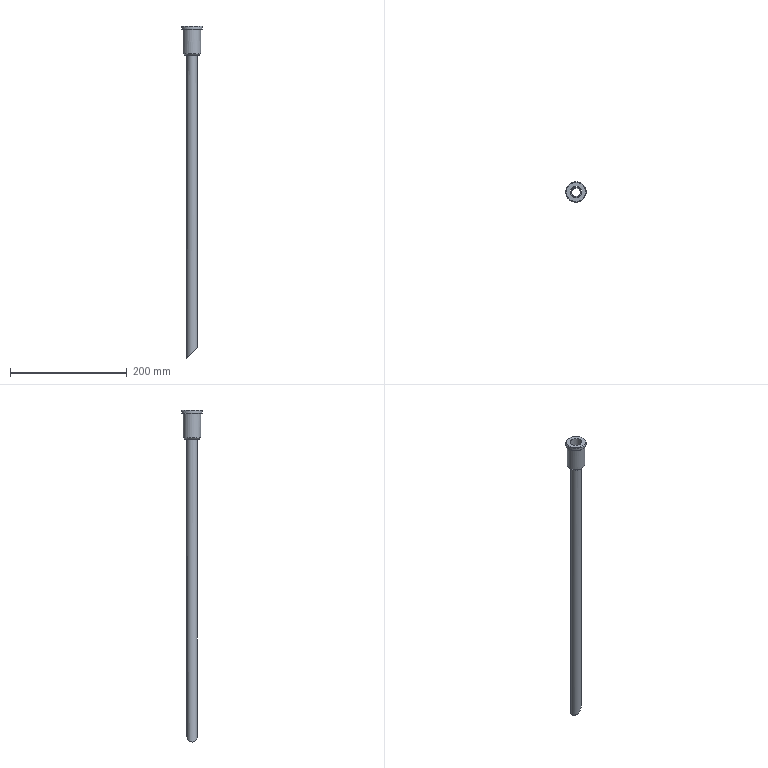Part | STEP file | HL4GZ-1.581.020 (return pipe weldment) | 2 solids | 14 faces | box 35 x 35 x 570 mm | volume 62212 mm3 | plane 5 | cylinder 5 | cone 3 | torus 1 | commonest cylinder face diameters 15 x1 18 x1 20 x1 30 x1 35 x1
STEP:
#1=CARTESIAN_POINT('',(0.,0.,0.));
#2=DIRECTION('',(0.,0.,1.));
#3=DIRECTION('',(1.,0.,0.));
#4=AXIS2_PLACEMENT_3D('',#1,#2,#3);
#5=CARTESIAN_POINT('',(1972.5,-700.,-232.5));
#6=VERTEX_POINT('',#5);
#7=CARTESIAN_POINT('',(1965.,-692.5,-240.));
#8=VERTEX_POINT('',#7);
#9=CARTESIAN_POINT('',(1965.,-700.,-240.));
#10=DIRECTION('',(0.7071,0.,-0.7071));
#11=DIRECTION('',(0.7071,0.,0.7071));
#12=AXIS2_PLACEMENT_3D('',#9,#10,#11);
#13=ELLIPSE('',#12,10.607,7.5);
#14=CARTESIAN_POINT('',(1970.142,-684.,-234.858));
#15=DIRECTION('',(0.7071,0.,-0.7071));
#16=DIRECTION('',(0.7071,0.,0.7071));
#17=AXIS2_PLACEMENT_3D('',#14,#15,#16);
#18=PLANE('',#17);
#19=CARTESIAN_POINT('',(-7.272,16.));
#20=DIRECTION('',(1.,0.));
#21=AXIS2_PLACEMENT_2D('',#19,#20);
#22=ELLIPSE('',#21,10.607,7.5);
#23=(GEOMETRIC_REPRESENTATION_CONTEXT(2)PARAMETRIC_REPRESENTATION_CONTEXT()REPRESENTATION_CONTEXT('',''));
#24=DEFINITIONAL_REPRESENTATION('',(#22),#23);
#25=PCURVE('',#18,#24);
#26=CARTESIAN_POINT('',(1965.,-700.,311.));
#27=DIRECTION('',(0.,0.,1.));
#28=DIRECTION('',(0.,1.,0.));
#29=AXIS2_PLACEMENT_3D('',#26,#27,#28);
#30=CYLINDRICAL_SURFACE('',#29,7.5);
#31=CARTESIAN_POINT('',(4.712,-543.5));
#32=CARTESIAN_POINT('',(4.617,-543.496));
#33=CARTESIAN_POINT('',(4.427,-543.707));
#34=CARTESIAN_POINT('',(4.141,-544.604));
#35=CARTESIAN_POINT('',(3.856,-546.021));
#36=CARTESIAN_POINT('',(3.57,-547.842));
#37=CARTESIAN_POINT('',(3.284,-549.918));
#38=CARTESIAN_POINT('',(2.999,-552.082));
#39=CARTESIAN_POINT('',(2.713,-554.158));
#40=CARTESIAN_POINT('',(2.428,-555.979));
#41=CARTESIAN_POINT('',(2.142,-557.396));
#42=CARTESIAN_POINT('',(1.856,-558.295));
#43=CARTESIAN_POINT('',(1.571,-558.603));
#44=CARTESIAN_POINT('',(1.285,-558.295));
#45=CARTESIAN_POINT('',(0.9996,-557.396));
#46=CARTESIAN_POINT('',(0.714,-555.979));
#47=CARTESIAN_POINT('',(0.4284,-554.158));
#48=CARTESIAN_POINT('',(0.1428,-552.082));
#49=CARTESIAN_POINT('',(-0.1428,-549.918));
#50=CARTESIAN_POINT('',(-0.4284,-547.842));
#51=CARTESIAN_POINT('',(-0.714,-546.021));
#52=CARTESIAN_POINT('',(-0.9996,-544.604));
#53=CARTESIAN_POINT('',(-1.285,-543.707));
#54=CARTESIAN_POINT('',(-1.476,-543.496));
#55=CARTESIAN_POINT('',(-1.571,-543.5));
#56=B_SPLINE_CURVE_WITH_KNOTS('',3,(#31,#32,#33,#34,#35,#36,#37,#38,#39,#40,#41,#42,#43,#44,#45,#46,#47,#48,#49,#50,#51,#52,#53,#54,#55),.UNSPECIFIED.,.F.,.F.,(4,1,1,1,1,1,1,1,1,1,1,1,1,1,1,1,1,1,1,1,1,1,4),(0.,0.2856,0.5712,0.8568,1.142,1.428,1.714,1.999,2.285,2.57,2.856,3.142,3.427,3.713,3.998,4.284,4.57,4.855,5.141,5.426,5.712,5.998,6.283),.QUASI_UNIFORM_KNOTS.);
#57=(GEOMETRIC_REPRESENTATION_CONTEXT(2)PARAMETRIC_REPRESENTATION_CONTEXT()REPRESENTATION_CONTEXT('',''));
#58=DEFINITIONAL_REPRESENTATION('',(#56),#57);
#59=PCURVE('',#30,#58);
#60=SURFACE_CURVE('',#13,(#25,#59),.PCURVE_S1.);
#61=EDGE_CURVE('',#6,#8,#60,.T.);
#62=ORIENTED_EDGE('',*,*,#61,.F.);
#63=CARTESIAN_POINT('',(1965.,-700.,-240.));
#64=DIRECTION('',(0.7071,0.,-0.7071));
#65=DIRECTION('',(0.7071,0.,0.7071));
#66=AXIS2_PLACEMENT_3D('',#63,#64,#65);
#67=ELLIPSE('',#66,10.607,7.5);
#68=CARTESIAN_POINT('',(-7.272,16.));
#69=DIRECTION('',(1.,0.));
#70=AXIS2_PLACEMENT_2D('',#68,#69);
#71=ELLIPSE('',#70,10.607,7.5);
#72=(GEOMETRIC_REPRESENTATION_CONTEXT(2)PARAMETRIC_REPRESENTATION_CONTEXT()REPRESENTATION_CONTEXT('',''));
#73=DEFINITIONAL_REPRESENTATION('',(#71),#72);
#74=PCURVE('',#18,#73);
#75=CARTESIAN_POINT('',(10.996,-543.5));
#76=CARTESIAN_POINT('',(10.9,-543.496));
#77=CARTESIAN_POINT('',(10.71,-543.707));
#78=CARTESIAN_POINT('',(10.424,-544.604));
#79=CARTESIAN_POINT('',(10.139,-546.021));
#80=CARTESIAN_POINT('',(9.853,-547.842));
#81=CARTESIAN_POINT('',(9.568,-549.918));
#82=CARTESIAN_POINT('',(9.282,-552.082));
#83=CARTESIAN_POINT('',(8.996,-554.158));
#84=CARTESIAN_POINT('',(8.711,-555.979));
#85=CARTESIAN_POINT('',(8.425,-557.396));
#86=CARTESIAN_POINT('',(8.14,-558.295));
#87=CARTESIAN_POINT('',(7.854,-558.603));
#88=CARTESIAN_POINT('',(7.568,-558.295));
#89=CARTESIAN_POINT('',(7.283,-557.396));
#90=CARTESIAN_POINT('',(6.997,-555.979));
#91=CARTESIAN_POINT('',(6.712,-554.158));
#92=CARTESIAN_POINT('',(6.426,-552.082));
#93=CARTESIAN_POINT('',(6.14,-549.918));
#94=CARTESIAN_POINT('',(5.855,-547.842));
#95=CARTESIAN_POINT('',(5.569,-546.021));
#96=CARTESIAN_POINT('',(5.284,-544.604));
#97=CARTESIAN_POINT('',(4.998,-543.707));
#98=CARTESIAN_POINT('',(4.808,-543.496));
#99=CARTESIAN_POINT('',(4.712,-543.5));
#100=B_SPLINE_CURVE_WITH_KNOTS('',3,(#75,#76,#77,#78,#79,#80,#81,#82,#83,#84,#85,#86,#87,#88,#89,#90,#91,#92,#93,#94,#95,#96,#97,#98,#99),.UNSPECIFIED.,.F.,.F.,(4,1,1,1,1,1,1,1,1,1,1,1,1,1,1,1,1,1,1,1,1,1,4),(0.,0.2856,0.5712,0.8568,1.142,1.428,1.714,1.999,2.285,2.57,2.856,3.142,3.427,3.713,3.998,4.284,4.57,4.855,5.141,5.426,5.712,5.998,6.283),.QUASI_UNIFORM_KNOTS.);
#101=(GEOMETRIC_REPRESENTATION_CONTEXT(2)PARAMETRIC_REPRESENTATION_CONTEXT()REPRESENTATION_CONTEXT('',''));
#102=DEFINITIONAL_REPRESENTATION('',(#100),#101);
#103=PCURVE('',#30,#102);
#104=SURFACE_CURVE('',#67,(#74,#103),.PCURVE_S1.);
#105=EDGE_CURVE('',#8,#6,#104,.T.);
#106=ORIENTED_EDGE('',*,*,#105,.F.);
#107=EDGE_LOOP('',(#62,#106));
#108=FACE_BOUND('',#107,.T.);
#109=CARTESIAN_POINT('',(1974.,-700.,-231.));
#110=VERTEX_POINT('',#109);
#111=CARTESIAN_POINT('',(1965.,-691.,-240.));
#112=VERTEX_POINT('',#111);
#113=CARTESIAN_POINT('',(1965.,-700.,-240.));
#114=DIRECTION('',(-0.7071,0.,0.7071));
#115=DIRECTION('',(0.7071,0.,0.7071));
#116=AXIS2_PLACEMENT_3D('',#113,#114,#115);
#117=ELLIPSE('',#116,12.728,9.);
#118=CARTESIAN_POINT('',(5.456,16.));
#119=CARTESIAN_POINT('',(5.456,0.4115));
#120=CARTESIAN_POINT('',(-13.636,8.206));
#121=CARTESIAN_POINT('',(-32.728,16.));
#122=CARTESIAN_POINT('',(-13.636,23.794));
#123=CARTESIAN_POINT('',(5.456,31.588));
#124=CARTESIAN_POINT('',(5.456,16.));
#125=(BOUNDED_CURVE()B_SPLINE_CURVE(2,(#118,#119,#120,#121,#122,#123,#124),.UNSPECIFIED.,.T.,.F.)B_SPLINE_CURVE_WITH_KNOTS((1,2,2,2,2,1),(-2.094,0.,2.094,4.189,6.283,8.378),.UNSPECIFIED.)CURVE()GEOMETRIC_REPRESENTATION_ITEM()RATIONAL_B_SPLINE_CURVE((1.,0.5,1.,0.5,1.,0.5,1.))REPRESENTATION_ITEM(''));
#126=(GEOMETRIC_REPRESENTATION_CONTEXT(2)PARAMETRIC_REPRESENTATION_CONTEXT()REPRESENTATION_CONTEXT('',''));
#127=DEFINITIONAL_REPRESENTATION('',(#125),#126);
#128=PCURVE('',#18,#127);
#129=CARTESIAN_POINT('',(1965.,-700.,311.));
#130=DIRECTION('',(0.,0.,1.));
#131=DIRECTION('',(0.,1.,0.));
#132=AXIS2_PLACEMENT_3D('',#129,#130,#131);
#133=CYLINDRICAL_SURFACE('',#132,9.);
#134=CARTESIAN_POINT('',(4.712,-542.));
#135=CARTESIAN_POINT('',(4.808,-541.995));
#136=CARTESIAN_POINT('',(4.998,-542.249));
#137=CARTESIAN_POINT('',(5.284,-543.325));
#138=CARTESIAN_POINT('',(5.569,-545.026));
#139=CARTESIAN_POINT('',(5.855,-547.21));
#140=CARTESIAN_POINT('',(6.14,-549.702));
#141=CARTESIAN_POINT('',(6.426,-552.298));
#142=CARTESIAN_POINT('',(6.712,-554.79));
#143=CARTESIAN_POINT('',(6.997,-556.974));
#144=CARTESIAN_POINT('',(7.283,-558.675));
#145=CARTESIAN_POINT('',(7.568,-559.754));
#146=CARTESIAN_POINT('',(7.854,-560.123));
#147=CARTESIAN_POINT('',(8.14,-559.754));
#148=CARTESIAN_POINT('',(8.425,-558.675));
#149=CARTESIAN_POINT('',(8.711,-556.974));
#150=CARTESIAN_POINT('',(8.996,-554.79));
#151=CARTESIAN_POINT('',(9.282,-552.298));
#152=CARTESIAN_POINT('',(9.568,-549.702));
#153=CARTESIAN_POINT('',(9.853,-547.21));
#154=CARTESIAN_POINT('',(10.139,-545.026));
#155=CARTESIAN_POINT('',(10.424,-543.325));
#156=CARTESIAN_POINT('',(10.71,-542.249));
#157=CARTESIAN_POINT('',(10.9,-541.995));
#158=CARTESIAN_POINT('',(10.996,-542.));
#159=B_SPLINE_CURVE_WITH_KNOTS('',3,(#134,#135,#136,#137,#138,#139,#140,#141,#142,#143,#144,#145,#146,#147,#148,#149,#150,#151,#152,#153,#154,#155,#156,#157,#158),.UNSPECIFIED.,.F.,.F.,(4,1,1,1,1,1,1,1,1,1,1,1,1,1,1,1,1,1,1,1,1,1,4),(0.,0.2856,0.5712,0.8568,1.142,1.428,1.714,1.999,2.285,2.57,2.856,3.142,3.427,3.713,3.998,4.284,4.57,4.855,5.141,5.426,5.712,5.998,6.283),.QUASI_UNIFORM_KNOTS.);
#160=(GEOMETRIC_REPRESENTATION_CONTEXT(2)PARAMETRIC_REPRESENTATION_CONTEXT()REPRESENTATION_CONTEXT('',''));
#161=DEFINITIONAL_REPRESENTATION('',(#159),#160);
#162=PCURVE('',#133,#161);
#163=SURFACE_CURVE('',#117,(#128,#162),.PCURVE_S1.);
#164=EDGE_CURVE('',#110,#112,#163,.T.);
#165=ORIENTED_EDGE('',*,*,#164,.F.);
#166=CARTESIAN_POINT('',(1965.,-700.,-240.));
#167=DIRECTION('',(-0.7071,0.,0.7071));
#168=DIRECTION('',(0.7071,0.,0.7071));
#169=AXIS2_PLACEMENT_3D('',#166,#167,#168);
#170=ELLIPSE('',#169,12.728,9.);
#171=CARTESIAN_POINT('',(5.456,16.));
#172=CARTESIAN_POINT('',(5.456,0.4115));
#173=CARTESIAN_POINT('',(-13.636,8.206));
#174=CARTESIAN_POINT('',(-32.728,16.));
#175=CARTESIAN_POINT('',(-13.636,23.794));
#176=CARTESIAN_POINT('',(5.456,31.588));
#177=CARTESIAN_POINT('',(5.456,16.));
#178=(BOUNDED_CURVE()B_SPLINE_CURVE(2,(#171,#172,#173,#174,#175,#176,#177),.UNSPECIFIED.,.T.,.F.)B_SPLINE_CURVE_WITH_KNOTS((1,2,2,2,2,1),(-2.094,0.,2.094,4.189,6.283,8.378),.UNSPECIFIED.)CURVE()GEOMETRIC_REPRESENTATION_ITEM()RATIONAL_B_SPLINE_CURVE((1.,0.5,1.,0.5,1.,0.5,1.))REPRESENTATION_ITEM(''));
#179=(GEOMETRIC_REPRESENTATION_CONTEXT(2)PARAMETRIC_REPRESENTATION_CONTEXT()REPRESENTATION_CONTEXT('',''));
#180=DEFINITIONAL_REPRESENTATION('',(#178),#179);
#181=PCURVE('',#18,#180);
#182=CARTESIAN_POINT('',(-1.571,-542.));
#183=CARTESIAN_POINT('',(-1.476,-541.995));
#184=CARTESIAN_POINT('',(-1.285,-542.249));
#185=CARTESIAN_POINT('',(-0.9996,-543.325));
#186=CARTESIAN_POINT('',(-0.714,-545.026));
#187=CARTESIAN_POINT('',(-0.4284,-547.21));
#188=CARTESIAN_POINT('',(-0.1428,-549.702));
#189=CARTESIAN_POINT('',(0.1428,-552.298));
#190=CARTESIAN_POINT('',(0.4284,-554.79));
#191=CARTESIAN_POINT('',(0.714,-556.974));
#192=CARTESIAN_POINT('',(0.9996,-558.675));
#193=CARTESIAN_POINT('',(1.285,-559.754));
#194=CARTESIAN_POINT('',(1.571,-560.123));
#195=CARTESIAN_POINT('',(1.856,-559.754));
#196=CARTESIAN_POINT('',(2.142,-558.675));
#197=CARTESIAN_POINT('',(2.428,-556.974));
#198=CARTESIAN_POINT('',(2.713,-554.79));
#199=CARTESIAN_POINT('',(2.999,-552.298));
#200=CARTESIAN_POINT('',(3.284,-549.702));
#201=CARTESIAN_POINT('',(3.57,-547.21));
#202=CARTESIAN_POINT('',(3.856,-545.026));
#203=CARTESIAN_POINT('',(4.141,-543.325));
#204=CARTESIAN_POINT('',(4.427,-542.249));
#205=CARTESIAN_POINT('',(4.617,-541.995));
#206=CARTESIAN_POINT('',(4.712,-542.));
#207=B_SPLINE_CURVE_WITH_KNOTS('',3,(#182,#183,#184,#185,#186,#187,#188,#189,#190,#191,#192,#193,#194,#195,#196,#197,#198,#199,#200,#201,#202,#203,#204,#205,#206),.UNSPECIFIED.,.F.,.F.,(4,1,1,1,1,1,1,1,1,1,1,1,1,1,1,1,1,1,1,1,1,1,4),(0.,0.2856,0.5712,0.8568,1.142,1.428,1.714,1.999,2.285,2.57,2.856,3.142,3.427,3.713,3.998,4.284,4.57,4.855,5.141,5.426,5.712,5.998,6.283),.QUASI_UNIFORM_KNOTS.);
#208=(GEOMETRIC_REPRESENTATION_CONTEXT(2)PARAMETRIC_REPRESENTATION_CONTEXT()REPRESENTATION_CONTEXT('',''));
#209=DEFINITIONAL_REPRESENTATION('',(#207),#208);
#210=PCURVE('',#133,#209);
#211=SURFACE_CURVE('',#170,(#181,#210),.PCURVE_S1.);
#212=EDGE_CURVE('',#112,#110,#211,.T.);
#213=ORIENTED_EDGE('',*,*,#212,.F.);
#214=EDGE_LOOP('',(#165,#213));
#215=FACE_BOUND('',#214,.T.);
#216=ADVANCED_FACE('',(#108,#215),#18,.T.);
#217=CARTESIAN_POINT('',(1965.,-692.5,291.));
#218=VERTEX_POINT('',#217);
#219=CARTESIAN_POINT('',(1965.,-700.,291.));
#220=DIRECTION('',(0.,0.,1.));
#221=DIRECTION('',(0.,1.,0.));
#222=AXIS2_PLACEMENT_3D('',#219,#220,#221);
#223=CIRCLE('',#222,7.5);
#224=CARTESIAN_POINT('',(1965.,-700.,291.));
#225=DIRECTION('',(0.,0.,-1.));
#226=DIRECTION('',(-1.,0.,0.));
#227=AXIS2_PLACEMENT_3D('',#224,#225,#226);
#228=PLANE('',#227);
#229=CARTESIAN_POINT('',(0.,7.5));
#230=CARTESIAN_POINT('',(12.99,7.5));
#231=CARTESIAN_POINT('',(6.495,-3.75));
#232=CARTESIAN_POINT('',(0.,-15.));
#233=CARTESIAN_POINT('',(-6.495,-3.75));
#234=CARTESIAN_POINT('',(-12.99,7.5));
#235=CARTESIAN_POINT('',(0.,7.5));
#236=(BOUNDED_CURVE()B_SPLINE_CURVE(2,(#229,#230,#231,#232,#233,#234,#235),.UNSPECIFIED.,.T.,.F.)B_SPLINE_CURVE_WITH_KNOTS((1,2,2,2,2,1),(-2.094,0.,2.094,4.189,6.283,8.378),.UNSPECIFIED.)CURVE()GEOMETRIC_REPRESENTATION_ITEM()RATIONAL_B_SPLINE_CURVE((1.,0.5,1.,0.5,1.,0.5,1.))REPRESENTATION_ITEM(''));
#237=(GEOMETRIC_REPRESENTATION_CONTEXT(2)PARAMETRIC_REPRESENTATION_CONTEXT()REPRESENTATION_CONTEXT('',''));
#238=DEFINITIONAL_REPRESENTATION('',(#236),#237);
#239=PCURVE('',#228,#238);
#240=CARTESIAN_POINT('',(0.,-20.));
#241=DIRECTION('',(1.,0.));
#242=VECTOR('',#241,1.);
#243=LINE('',#240,#242);
#244=(GEOMETRIC_REPRESENTATION_CONTEXT(2)PARAMETRIC_REPRESENTATION_CONTEXT()REPRESENTATION_CONTEXT('',''));
#245=DEFINITIONAL_REPRESENTATION('',(#243),#244);
#246=PCURVE('',#30,#245);
#247=SURFACE_CURVE('',#223,(#239,#246),.PCURVE_S1.);
#248=EDGE_CURVE('',#218,#218,#247,.T.);
#249=ORIENTED_EDGE('',*,*,#248,.F.);
#250=EDGE_LOOP('',(#249));
#251=FACE_BOUND('',#250,.T.);
#252=CARTESIAN_POINT('',(1965.,-691.,291.));
#253=VERTEX_POINT('',#252);
#254=CARTESIAN_POINT('',(1965.,-700.,291.));
#255=DIRECTION('',(0.,0.,-1.));
#256=DIRECTION('',(0.,1.,0.));
#257=AXIS2_PLACEMENT_3D('',#254,#255,#256);
#258=CIRCLE('',#257,9.);
#259=CARTESIAN_POINT('',(0.,0.));
#260=DIRECTION('',(0.,1.));
#261=AXIS2_PLACEMENT_2D('',#259,#260);
#262=CIRCLE('',#261,9.);
#263=(GEOMETRIC_REPRESENTATION_CONTEXT(2)PARAMETRIC_REPRESENTATION_CONTEXT()REPRESENTATION_CONTEXT('',''));
#264=DEFINITIONAL_REPRESENTATION('',(#262),#263);
#265=PCURVE('',#228,#264);
#266=CARTESIAN_POINT('',(6.283,-20.));
#267=DIRECTION('',(-1.,0.));
#268=VECTOR('',#267,1.);
#269=LINE('',#266,#268);
#270=(GEOMETRIC_REPRESENTATION_CONTEXT(2)PARAMETRIC_REPRESENTATION_CONTEXT()REPRESENTATION_CONTEXT('',''));
#271=DEFINITIONAL_REPRESENTATION('',(#269),#270);
#272=PCURVE('',#133,#271);
#273=SURFACE_CURVE('',#258,(#265,#272),.PCURVE_S1.);
#274=EDGE_CURVE('',#253,#253,#273,.T.);
#275=ORIENTED_EDGE('',*,*,#274,.F.);
#276=EDGE_LOOP('',(#275));
#277=FACE_BOUND('',#276,.T.);
#278=ADVANCED_FACE('',(#251,#277),#228,.F.);
#279=ORIENTED_EDGE('',*,*,#105,.F.);
#280=CARTESIAN_POINT('',(1965.,-692.5,-240.));
#281=CARTESIAN_POINT('',(1965.,-692.5,291.));
#282=B_SPLINE_CURVE_WITH_KNOTS('',1,(#280,#281),.UNSPECIFIED.,.F.,.F.,(2,2),(-551.,-20.),.PIECEWISE_BEZIER_KNOTS.);
#283=CARTESIAN_POINT('',(6.283,0.));
#284=DIRECTION('',(0.,1.));
#285=VECTOR('',#284,1.);
#286=LINE('',#283,#285);
#287=(GEOMETRIC_REPRESENTATION_CONTEXT(2)PARAMETRIC_REPRESENTATION_CONTEXT()REPRESENTATION_CONTEXT('',''));
#288=DEFINITIONAL_REPRESENTATION('',(#286),#287);
#289=PCURVE('',#30,#288);
#290=CARTESIAN_POINT('',(0.,0.));
#291=DIRECTION('',(0.,1.));
#292=VECTOR('',#291,1.);
#293=LINE('',#290,#292);
#294=(GEOMETRIC_REPRESENTATION_CONTEXT(2)PARAMETRIC_REPRESENTATION_CONTEXT()REPRESENTATION_CONTEXT('',''));
#295=DEFINITIONAL_REPRESENTATION('',(#293),#294);
#296=PCURVE('',#30,#295);
#297=SEAM_CURVE('',#282,(#289,#296),.PCURVE_S1.);
#298=EDGE_CURVE('',#8,#218,#297,.T.);
#299=ORIENTED_EDGE('',*,*,#298,.T.);
#300=ORIENTED_EDGE('',*,*,#248,.F.);
#301=ORIENTED_EDGE('',*,*,#298,.F.);
#302=ORIENTED_EDGE('',*,*,#61,.F.);
#303=EDGE_LOOP('',(#279,#299,#300,#301,#302));
#304=FACE_BOUND('',#303,.F.);
#305=ADVANCED_FACE('',(#304),#30,.F.);
#306=ORIENTED_EDGE('',*,*,#164,.T.);
#307=CARTESIAN_POINT('',(1965.,-691.,-240.));
#308=CARTESIAN_POINT('',(1965.,-691.,291.));
#309=B_SPLINE_CURVE_WITH_KNOTS('',1,(#307,#308),.UNSPECIFIED.,.F.,.F.,(2,2),(-551.,-20.),.PIECEWISE_BEZIER_KNOTS.);
#310=CARTESIAN_POINT('',(6.283,0.));
#311=DIRECTION('',(0.,1.));
#312=VECTOR('',#311,1.);
#313=LINE('',#310,#312);
#314=(GEOMETRIC_REPRESENTATION_CONTEXT(2)PARAMETRIC_REPRESENTATION_CONTEXT()REPRESENTATION_CONTEXT('',''));
#315=DEFINITIONAL_REPRESENTATION('',(#313),#314);
#316=PCURVE('',#133,#315);
#317=CARTESIAN_POINT('',(0.,0.));
#318=DIRECTION('',(0.,1.));
#319=VECTOR('',#318,1.);
#320=LINE('',#317,#319);
#321=(GEOMETRIC_REPRESENTATION_CONTEXT(2)PARAMETRIC_REPRESENTATION_CONTEXT()REPRESENTATION_CONTEXT('',''));
#322=DEFINITIONAL_REPRESENTATION('',(#320),#321);
#323=PCURVE('',#133,#322);
#324=SEAM_CURVE('',#309,(#316,#323),.PCURVE_S1.);
#325=EDGE_CURVE('',#112,#253,#324,.T.);
#326=ORIENTED_EDGE('',*,*,#325,.T.);
#327=ORIENTED_EDGE('',*,*,#274,.T.);
#328=ORIENTED_EDGE('',*,*,#325,.F.);
#329=ORIENTED_EDGE('',*,*,#212,.T.);
#330=EDGE_LOOP('',(#306,#326,#327,#328,#329));
#331=FACE_BOUND('',#330,.T.);
#332=ADVANCED_FACE('',(#331),#133,.T.);
#333=CLOSED_SHELL('',(#216,#278,#305,#332));
#334=MANIFOLD_SOLID_BREP('',#333);
#335=CARTESIAN_POINT('',(1950.,-700.,273.));
#336=VERTEX_POINT('',#335);
#337=CARTESIAN_POINT('',(1980.,-700.,273.));
#338=VERTEX_POINT('',#337);
#339=CARTESIAN_POINT('',(1965.,-700.,273.));
#340=DIRECTION('',(0.,0.,1.));
#341=DIRECTION('',(1.,0.,0.));
#342=AXIS2_PLACEMENT_3D('',#339,#340,#341);
#343=CIRCLE('',#342,15.);
#344=CARTESIAN_POINT('',(1965.,-700.,273.));
#345=DIRECTION('',(0.,0.,1.));
#346=DIRECTION('',(-1.,0.,0.));
#347=AXIS2_PLACEMENT_3D('',#344,#345,#346);
#348=CONICAL_SURFACE('',#347,15.,0.7854);
#349=CARTESIAN_POINT('',(-3.142,0.));
#350=DIRECTION('',(1.,0.));
#351=VECTOR('',#350,1.);
#352=LINE('',#349,#351);
#353=(GEOMETRIC_REPRESENTATION_CONTEXT(2)PARAMETRIC_REPRESENTATION_CONTEXT()REPRESENTATION_CONTEXT('',''));
#354=DEFINITIONAL_REPRESENTATION('',(#352),#353);
#355=PCURVE('',#348,#354);
#356=CARTESIAN_POINT('',(1965.,-700.,315.));
#357=DIRECTION('',(0.,0.,-1.));
#358=DIRECTION('',(-1.,0.,0.));
#359=AXIS2_PLACEMENT_3D('',#356,#357,#358);
#360=CYLINDRICAL_SURFACE('',#359,15.);
#361=CARTESIAN_POINT('',(9.425,42.));
#362=DIRECTION('',(-1.,0.));
#363=VECTOR('',#362,1.);
#364=LINE('',#361,#363);
#365=(GEOMETRIC_REPRESENTATION_CONTEXT(2)PARAMETRIC_REPRESENTATION_CONTEXT()REPRESENTATION_CONTEXT('',''));
#366=DEFINITIONAL_REPRESENTATION('',(#364),#365);
#367=PCURVE('',#360,#366);
#368=SURFACE_CURVE('',#343,(#355,#367),.PCURVE_S1.);
#369=EDGE_CURVE('',#336,#338,#368,.T.);
#370=ORIENTED_EDGE('',*,*,#369,.F.);
#371=CARTESIAN_POINT('',(1952.,-700.,271.));
#372=VERTEX_POINT('',#371);
#373=CARTESIAN_POINT('',(1952.,-700.,271.));
#374=CARTESIAN_POINT('',(1950.,-700.,273.));
#375=B_SPLINE_CURVE_WITH_KNOTS('',1,(#373,#374),.UNSPECIFIED.,.F.,.F.,(2,2),(-2.828,0.),.PIECEWISE_BEZIER_KNOTS.);
#376=CARTESIAN_POINT('',(0.,0.));
#377=DIRECTION('',(0.,1.));
#378=VECTOR('',#377,1.);
#379=LINE('',#376,#378);
#380=(GEOMETRIC_REPRESENTATION_CONTEXT(2)PARAMETRIC_REPRESENTATION_CONTEXT()REPRESENTATION_CONTEXT('',''));
#381=DEFINITIONAL_REPRESENTATION('',(#379),#380);
#382=PCURVE('',#348,#381);
#383=CARTESIAN_POINT('',(6.283,0.));
#384=DIRECTION('',(0.,1.));
#385=VECTOR('',#384,1.);
#386=LINE('',#383,#385);
#387=(GEOMETRIC_REPRESENTATION_CONTEXT(2)PARAMETRIC_REPRESENTATION_CONTEXT()REPRESENTATION_CONTEXT('',''));
#388=DEFINITIONAL_REPRESENTATION('',(#386),#387);
#389=PCURVE('',#348,#388);
#390=SEAM_CURVE('',#375,(#382,#389),.PCURVE_S1.);
#391=EDGE_CURVE('',#372,#336,#390,.T.);
#392=ORIENTED_EDGE('',*,*,#391,.F.);
#393=CARTESIAN_POINT('',(1965.,-700.,271.));
#394=DIRECTION('',(0.,0.,-1.));
#395=DIRECTION('',(-1.,0.,0.));
#396=AXIS2_PLACEMENT_3D('',#393,#394,#395);
#397=CIRCLE('',#396,13.);
#398=CARTESIAN_POINT('',(6.283,-2.));
#399=DIRECTION('',(-1.,0.));
#400=VECTOR('',#399,1.);
#401=LINE('',#398,#400);
#402=(GEOMETRIC_REPRESENTATION_CONTEXT(2)PARAMETRIC_REPRESENTATION_CONTEXT()REPRESENTATION_CONTEXT('',''));
#403=DEFINITIONAL_REPRESENTATION('',(#401),#402);
#404=PCURVE('',#348,#403);
#405=CARTESIAN_POINT('',(1965.,-700.,271.));
#406=DIRECTION('',(0.,0.,-1.));
#407=DIRECTION('',(-1.,0.,0.));
#408=AXIS2_PLACEMENT_3D('',#405,#406,#407);
#409=PLANE('',#408);
#410=CARTESIAN_POINT('',(0.,0.));
#411=DIRECTION('',(1.,0.));
#412=AXIS2_PLACEMENT_2D('',#410,#411);
#413=CIRCLE('',#412,13.);
#414=(GEOMETRIC_REPRESENTATION_CONTEXT(2)PARAMETRIC_REPRESENTATION_CONTEXT()REPRESENTATION_CONTEXT('',''));
#415=DEFINITIONAL_REPRESENTATION('',(#413),#414);
#416=PCURVE('',#409,#415);
#417=SURFACE_CURVE('',#397,(#404,#416),.PCURVE_S1.);
#418=EDGE_CURVE('',#372,#372,#417,.T.);
#419=ORIENTED_EDGE('',*,*,#418,.F.);
#420=ORIENTED_EDGE('',*,*,#391,.T.);
#421=CARTESIAN_POINT('',(1965.,-700.,273.));
#422=DIRECTION('',(0.,0.,1.));
#423=DIRECTION('',(1.,0.,0.));
#424=AXIS2_PLACEMENT_3D('',#421,#422,#423);
#425=CIRCLE('',#424,15.);
#426=CARTESIAN_POINT('',(3.142,0.));
#427=DIRECTION('',(1.,0.));
#428=VECTOR('',#427,1.);
#429=LINE('',#426,#428);
#430=(GEOMETRIC_REPRESENTATION_CONTEXT(2)PARAMETRIC_REPRESENTATION_CONTEXT()REPRESENTATION_CONTEXT('',''));
#431=DEFINITIONAL_REPRESENTATION('',(#429),#430);
#432=PCURVE('',#348,#431);
#433=CARTESIAN_POINT('',(3.142,42.));
#434=DIRECTION('',(-1.,0.));
#435=VECTOR('',#434,1.);
#436=LINE('',#433,#435);
#437=(GEOMETRIC_REPRESENTATION_CONTEXT(2)PARAMETRIC_REPRESENTATION_CONTEXT()REPRESENTATION_CONTEXT('',''));
#438=DEFINITIONAL_REPRESENTATION('',(#436),#437);
#439=PCURVE('',#360,#438);
#440=SURFACE_CURVE('',#425,(#432,#439),.PCURVE_S1.);
#441=EDGE_CURVE('',#338,#336,#440,.T.);
#442=ORIENTED_EDGE('',*,*,#441,.F.);
#443=EDGE_LOOP('',(#370,#392,#419,#420,#442));
#444=FACE_BOUND('',#443,.T.);
#445=ADVANCED_FACE('',(#444),#348,.T.);
#446=CARTESIAN_POINT('',(1965.,-690.,271.));
#447=VERTEX_POINT('',#446);
#448=CARTESIAN_POINT('',(1965.,-710.,271.));
#449=VERTEX_POINT('',#448);
#450=CARTESIAN_POINT('',(1965.,-700.,271.));
#451=DIRECTION('',(0.,0.,1.));
#452=DIRECTION('',(0.,1.,0.));
#453=AXIS2_PLACEMENT_3D('',#450,#451,#452);
#454=CIRCLE('',#453,10.);
#455=CARTESIAN_POINT('',(0.,10.));
#456=CARTESIAN_POINT('',(17.321,10.));
#457=CARTESIAN_POINT('',(8.66,-5.));
#458=CARTESIAN_POINT('',(0.,-20.));
#459=CARTESIAN_POINT('',(-8.66,-5.));
#460=CARTESIAN_POINT('',(-17.321,10.));
#461=CARTESIAN_POINT('',(0.,10.));
#462=(BOUNDED_CURVE()B_SPLINE_CURVE(2,(#455,#456,#457,#458,#459,#460,#461),.UNSPECIFIED.,.T.,.F.)B_SPLINE_CURVE_WITH_KNOTS((1,2,2,2,2,1),(-2.094,0.,2.094,4.189,6.283,8.378),.UNSPECIFIED.)CURVE()GEOMETRIC_REPRESENTATION_ITEM()RATIONAL_B_SPLINE_CURVE((1.,0.5,1.,0.5,1.,0.5,1.))REPRESENTATION_ITEM(''));
#463=(GEOMETRIC_REPRESENTATION_CONTEXT(2)PARAMETRIC_REPRESENTATION_CONTEXT()REPRESENTATION_CONTEXT('',''));
#464=DEFINITIONAL_REPRESENTATION('',(#462),#463);
#465=PCURVE('',#409,#464);
#466=CARTESIAN_POINT('',(1965.,-700.,325.));
#467=DIRECTION('',(0.,0.,-1.));
#468=DIRECTION('',(-1.,0.,0.));
#469=AXIS2_PLACEMENT_3D('',#466,#467,#468);
#470=CYLINDRICAL_SURFACE('',#469,10.);
#471=CARTESIAN_POINT('',(7.854,54.));
#472=DIRECTION('',(-1.,0.));
#473=VECTOR('',#472,1.);
#474=LINE('',#471,#473);
#475=(GEOMETRIC_REPRESENTATION_CONTEXT(2)PARAMETRIC_REPRESENTATION_CONTEXT()REPRESENTATION_CONTEXT('',''));
#476=DEFINITIONAL_REPRESENTATION('',(#474),#475);
#477=PCURVE('',#470,#476);
#478=SURFACE_CURVE('',#454,(#465,#477),.PCURVE_S1.);
#479=EDGE_CURVE('',#447,#449,#478,.T.);
#480=ORIENTED_EDGE('',*,*,#479,.T.);
#481=CARTESIAN_POINT('',(1965.,-700.,271.));
#482=DIRECTION('',(0.,0.,1.));
#483=DIRECTION('',(0.,1.,0.));
#484=AXIS2_PLACEMENT_3D('',#481,#482,#483);
#485=CIRCLE('',#484,10.);
#486=CARTESIAN_POINT('',(0.,10.));
#487=CARTESIAN_POINT('',(17.321,10.));
#488=CARTESIAN_POINT('',(8.66,-5.));
#489=CARTESIAN_POINT('',(0.,-20.));
#490=CARTESIAN_POINT('',(-8.66,-5.));
#491=CARTESIAN_POINT('',(-17.321,10.));
#492=CARTESIAN_POINT('',(0.,10.));
#493=(BOUNDED_CURVE()B_SPLINE_CURVE(2,(#486,#487,#488,#489,#490,#491,#492),.UNSPECIFIED.,.T.,.F.)B_SPLINE_CURVE_WITH_KNOTS((1,2,2,2,2,1),(-2.094,0.,2.094,4.189,6.283,8.378),.UNSPECIFIED.)CURVE()GEOMETRIC_REPRESENTATION_ITEM()RATIONAL_B_SPLINE_CURVE((1.,0.5,1.,0.5,1.,0.5,1.))REPRESENTATION_ITEM(''));
#494=(GEOMETRIC_REPRESENTATION_CONTEXT(2)PARAMETRIC_REPRESENTATION_CONTEXT()REPRESENTATION_CONTEXT('',''));
#495=DEFINITIONAL_REPRESENTATION('',(#493),#494);
#496=PCURVE('',#409,#495);
#497=CARTESIAN_POINT('',(14.137,54.));
#498=DIRECTION('',(-1.,0.));
#499=VECTOR('',#498,1.);
#500=LINE('',#497,#499);
#501=(GEOMETRIC_REPRESENTATION_CONTEXT(2)PARAMETRIC_REPRESENTATION_CONTEXT()REPRESENTATION_CONTEXT('',''));
#502=DEFINITIONAL_REPRESENTATION('',(#500),#501);
#503=PCURVE('',#470,#502);
#504=SURFACE_CURVE('',#485,(#496,#503),.PCURVE_S1.);
#505=EDGE_CURVE('',#449,#447,#504,.T.);
#506=ORIENTED_EDGE('',*,*,#505,.T.);
#507=EDGE_LOOP('',(#480,#506));
#508=FACE_BOUND('',#507,.T.);
#509=ORIENTED_EDGE('',*,*,#418,.T.);
#510=EDGE_LOOP('',(#509));
#511=FACE_BOUND('',#510,.T.);
#512=ADVANCED_FACE('',(#508,#511),#409,.T.);
#513=CARTESIAN_POINT('',(1965.,-717.,315.));
#514=VERTEX_POINT('',#513);
#515=CARTESIAN_POINT('',(1965.,-700.,315.));
#516=DIRECTION('',(0.,0.,-1.));
#517=DIRECTION('',(0.,-1.,0.));
#518=AXIS2_PLACEMENT_3D('',#515,#516,#517);
#519=CIRCLE('',#518,17.);
#520=CARTESIAN_POINT('',(1965.,-700.,315.));
#521=DIRECTION('',(0.,0.,1.));
#522=DIRECTION('',(0.,-1.,0.));
#523=AXIS2_PLACEMENT_3D('',#520,#521,#522);
#524=CONICAL_SURFACE('',#523,17.,0.7854);
#525=CARTESIAN_POINT('',(6.283,0.));
#526=DIRECTION('',(-1.,0.));
#527=VECTOR('',#526,1.);
#528=LINE('',#525,#527);
#529=(GEOMETRIC_REPRESENTATION_CONTEXT(2)PARAMETRIC_REPRESENTATION_CONTEXT()REPRESENTATION_CONTEXT('',''));
#530=DEFINITIONAL_REPRESENTATION('',(#528),#529);
#531=PCURVE('',#524,#530);
#532=CARTESIAN_POINT('',(1965.,-700.,315.));
#533=DIRECTION('',(0.,0.,-1.));
#534=DIRECTION('',(-1.,0.,0.));
#535=AXIS2_PLACEMENT_3D('',#532,#533,#534);
#536=PLANE('',#535);
#537=CARTESIAN_POINT('',(0.,0.));
#538=DIRECTION('',(0.,-1.));
#539=AXIS2_PLACEMENT_2D('',#537,#538);
#540=CIRCLE('',#539,17.);
#541=(GEOMETRIC_REPRESENTATION_CONTEXT(2)PARAMETRIC_REPRESENTATION_CONTEXT()REPRESENTATION_CONTEXT('',''));
#542=DEFINITIONAL_REPRESENTATION('',(#540),#541);
#543=PCURVE('',#536,#542);
#544=SURFACE_CURVE('',#519,(#531,#543),.PCURVE_S1.);
#545=EDGE_CURVE('',#514,#514,#544,.T.);
#546=ORIENTED_EDGE('',*,*,#545,.F.);
#547=CARTESIAN_POINT('',(1965.,-717.5,315.5));
#548=VERTEX_POINT('',#547);
#549=CARTESIAN_POINT('',(1965.,-717.,315.));
#550=CARTESIAN_POINT('',(1965.,-717.5,315.5));
#551=B_SPLINE_CURVE_WITH_KNOTS('',1,(#549,#550),.UNSPECIFIED.,.F.,.F.,(2,2),(0.,0.7071),.PIECEWISE_BEZIER_KNOTS.);
#552=CARTESIAN_POINT('',(6.283,0.));
#553=DIRECTION('',(0.,1.));
#554=VECTOR('',#553,1.);
#555=LINE('',#552,#554);
#556=(GEOMETRIC_REPRESENTATION_CONTEXT(2)PARAMETRIC_REPRESENTATION_CONTEXT()REPRESENTATION_CONTEXT('',''));
#557=DEFINITIONAL_REPRESENTATION('',(#555),#556);
#558=PCURVE('',#524,#557);
#559=CARTESIAN_POINT('',(0.,0.));
#560=DIRECTION('',(0.,1.));
#561=VECTOR('',#560,1.);
#562=LINE('',#559,#561);
#563=(GEOMETRIC_REPRESENTATION_CONTEXT(2)PARAMETRIC_REPRESENTATION_CONTEXT()REPRESENTATION_CONTEXT('',''));
#564=DEFINITIONAL_REPRESENTATION('',(#562),#563);
#565=PCURVE('',#524,#564);
#566=SEAM_CURVE('',#551,(#558,#565),.PCURVE_S1.);
#567=EDGE_CURVE('',#514,#548,#566,.T.);
#568=ORIENTED_EDGE('',*,*,#567,.T.);
#569=CARTESIAN_POINT('',(1965.,-682.5,315.5));
#570=VERTEX_POINT('',#569);
#571=CARTESIAN_POINT('',(1965.,-700.,315.5));
#572=DIRECTION('',(0.,0.,1.));
#573=DIRECTION('',(0.,1.,0.));
#574=AXIS2_PLACEMENT_3D('',#571,#572,#573);
#575=CIRCLE('',#574,17.5);
#576=CARTESIAN_POINT('',(3.142,0.5));
#577=DIRECTION('',(1.,0.));
#578=VECTOR('',#577,1.);
#579=LINE('',#576,#578);
#580=(GEOMETRIC_REPRESENTATION_CONTEXT(2)PARAMETRIC_REPRESENTATION_CONTEXT()REPRESENTATION_CONTEXT('',''));
#581=DEFINITIONAL_REPRESENTATION('',(#579),#580);
#582=PCURVE('',#524,#581);
#583=CARTESIAN_POINT('',(1965.,-700.,315.));
#584=DIRECTION('',(0.,0.,1.));
#585=DIRECTION('',(0.,1.,0.));
#586=AXIS2_PLACEMENT_3D('',#583,#584,#585);
#587=CYLINDRICAL_SURFACE('',#586,17.5);
#588=CARTESIAN_POINT('',(0.,0.5));
#589=DIRECTION('',(1.,0.));
#590=VECTOR('',#589,1.);
#591=LINE('',#588,#590);
#592=(GEOMETRIC_REPRESENTATION_CONTEXT(2)PARAMETRIC_REPRESENTATION_CONTEXT()REPRESENTATION_CONTEXT('',''));
#593=DEFINITIONAL_REPRESENTATION('',(#591),#592);
#594=PCURVE('',#587,#593);
#595=SURFACE_CURVE('',#575,(#582,#594),.PCURVE_S1.);
#596=EDGE_CURVE('',#570,#548,#595,.T.);
#597=ORIENTED_EDGE('',*,*,#596,.F.);
#598=CARTESIAN_POINT('',(1965.,-700.,315.5));
#599=DIRECTION('',(0.,0.,1.));
#600=DIRECTION('',(0.,1.,0.));
#601=AXIS2_PLACEMENT_3D('',#598,#599,#600);
#602=CIRCLE('',#601,17.5);
#603=CARTESIAN_POINT('',(-3.142,0.5));
#604=DIRECTION('',(1.,0.));
#605=VECTOR('',#604,1.);
#606=LINE('',#603,#605);
#607=(GEOMETRIC_REPRESENTATION_CONTEXT(2)PARAMETRIC_REPRESENTATION_CONTEXT()REPRESENTATION_CONTEXT('',''));
#608=DEFINITIONAL_REPRESENTATION('',(#606),#607);
#609=PCURVE('',#524,#608);
#610=CARTESIAN_POINT('',(0.,0.5));
#611=DIRECTION('',(1.,0.));
#612=VECTOR('',#611,1.);
#613=LINE('',#610,#612);
#614=(GEOMETRIC_REPRESENTATION_CONTEXT(2)PARAMETRIC_REPRESENTATION_CONTEXT()REPRESENTATION_CONTEXT('',''));
#615=DEFINITIONAL_REPRESENTATION('',(#613),#614);
#616=PCURVE('',#587,#615);
#617=SURFACE_CURVE('',#602,(#609,#616),.PCURVE_S1.);
#618=EDGE_CURVE('',#548,#570,#617,.T.);
#619=ORIENTED_EDGE('',*,*,#618,.F.);
#620=ORIENTED_EDGE('',*,*,#567,.F.);
#621=EDGE_LOOP('',(#546,#568,#597,#619,#620));
#622=FACE_BOUND('',#621,.T.);
#623=ADVANCED_FACE('',(#622),#524,.T.);
#624=CARTESIAN_POINT('',(1965.,-715.,314.5));
#625=VERTEX_POINT('',#624);
#626=CARTESIAN_POINT('',(1950.,-700.,314.5));
#627=VERTEX_POINT('',#626);
#628=CARTESIAN_POINT('',(1965.,-700.,314.5));
#629=DIRECTION('',(0.,0.,-1.));
#630=DIRECTION('',(0.,-1.,0.));
#631=AXIS2_PLACEMENT_3D('',#628,#629,#630);
#632=CIRCLE('',#631,15.);
#633=CARTESIAN_POINT('',(1965.,-700.,314.5));
#634=DIRECTION('',(0.,0.,-1.));
#635=DIRECTION('',(0.,1.,0.));
#636=AXIS2_PLACEMENT_3D('',#633,#634,#635);
#637=TOROIDAL_SURFACE('',#636,15.5,0.5);
#638=CARTESIAN_POINT('',(3.142,3.142));
#639=DIRECTION('',(1.,0.));
#640=VECTOR('',#639,1.);
#641=LINE('',#638,#640);
#642=(GEOMETRIC_REPRESENTATION_CONTEXT(2)PARAMETRIC_REPRESENTATION_CONTEXT()REPRESENTATION_CONTEXT('',''));
#643=DEFINITIONAL_REPRESENTATION('',(#641),#642);
#644=PCURVE('',#637,#643);
#645=CARTESIAN_POINT('',(4.712,0.5));
#646=DIRECTION('',(1.,0.));
#647=VECTOR('',#646,1.);
#648=LINE('',#645,#647);
#649=(GEOMETRIC_REPRESENTATION_CONTEXT(2)PARAMETRIC_REPRESENTATION_CONTEXT()REPRESENTATION_CONTEXT('',''));
#650=DEFINITIONAL_REPRESENTATION('',(#648),#649);
#651=PCURVE('',#360,#650);
#652=SURFACE_CURVE('',#632,(#644,#651),.PCURVE_S1.);
#653=EDGE_CURVE('',#625,#627,#652,.T.);
#654=ORIENTED_EDGE('',*,*,#653,.T.);
#655=CARTESIAN_POINT('',(1965.,-700.,314.5));
#656=DIRECTION('',(0.,0.,-1.));
#657=DIRECTION('',(0.,-1.,0.));
#658=AXIS2_PLACEMENT_3D('',#655,#656,#657);
#659=CIRCLE('',#658,15.);
#660=CARTESIAN_POINT('',(3.142,3.142));
#661=DIRECTION('',(1.,0.));
#662=VECTOR('',#661,1.);
#663=LINE('',#660,#662);
#664=(GEOMETRIC_REPRESENTATION_CONTEXT(2)PARAMETRIC_REPRESENTATION_CONTEXT()REPRESENTATION_CONTEXT('',''));
#665=DEFINITIONAL_REPRESENTATION('',(#663),#664);
#666=PCURVE('',#637,#665);
#667=CARTESIAN_POINT('',(-1.571,0.5));
#668=DIRECTION('',(1.,0.));
#669=VECTOR('',#668,1.);
#670=LINE('',#667,#669);
#671=(GEOMETRIC_REPRESENTATION_CONTEXT(2)PARAMETRIC_REPRESENTATION_CONTEXT()REPRESENTATION_CONTEXT('',''));
#672=DEFINITIONAL_REPRESENTATION('',(#670),#671);
#673=PCURVE('',#360,#672);
#674=SURFACE_CURVE('',#659,(#666,#673),.PCURVE_S1.);
#675=EDGE_CURVE('',#627,#625,#674,.T.);
#676=ORIENTED_EDGE('',*,*,#675,.T.);
#677=CARTESIAN_POINT('',(1965.,-715.5,315.));
#678=VERTEX_POINT('',#677);
#679=CARTESIAN_POINT('',(1965.,-715.,314.5));
#680=CARTESIAN_POINT('',(1965.,-715.,314.634));
#681=CARTESIAN_POINT('',(1965.,-715.042,314.764));
#682=CARTESIAN_POINT('',(1965.,-715.124,314.876));
#683=CARTESIAN_POINT('',(1965.,-715.236,314.958));
#684=CARTESIAN_POINT('',(1965.,-715.366,315.));
#685=CARTESIAN_POINT('',(1965.,-715.5,315.));
#686=(BOUNDED_CURVE()B_SPLINE_CURVE(6,(#679,#680,#681,#682,#683,#684,#685),.UNSPECIFIED.,.F.,.F.)B_SPLINE_CURVE_WITH_KNOTS((7,7),(3.142,4.712),.PIECEWISE_BEZIER_KNOTS.)CURVE()GEOMETRIC_REPRESENTATION_ITEM()RATIONAL_B_SPLINE_CURVE((1.031,1.01,0.9979,0.994,0.9979,1.01,1.031))REPRESENTATION_ITEM(''));
#687=CARTESIAN_POINT('',(9.425,0.));
#688=DIRECTION('',(0.,1.));
#689=VECTOR('',#688,1.);
#690=LINE('',#687,#689);
#691=(GEOMETRIC_REPRESENTATION_CONTEXT(2)PARAMETRIC_REPRESENTATION_CONTEXT()REPRESENTATION_CONTEXT('',''));
#692=DEFINITIONAL_REPRESENTATION('',(#690),#691);
#693=PCURVE('',#637,#692);
#694=CARTESIAN_POINT('',(3.142,0.));
#695=DIRECTION('',(0.,1.));
#696=VECTOR('',#695,1.);
#697=LINE('',#694,#696);
#698=(GEOMETRIC_REPRESENTATION_CONTEXT(2)PARAMETRIC_REPRESENTATION_CONTEXT()REPRESENTATION_CONTEXT('',''));
#699=DEFINITIONAL_REPRESENTATION('',(#697),#698);
#700=PCURVE('',#637,#699);
#701=SEAM_CURVE('',#686,(#693,#700),.PCURVE_S1.);
#702=EDGE_CURVE('',#625,#678,#701,.T.);
#703=ORIENTED_EDGE('',*,*,#702,.T.);
#704=CARTESIAN_POINT('',(1965.,-700.,315.));
#705=DIRECTION('',(0.,0.,1.));
#706=DIRECTION('',(0.,-1.,0.));
#707=AXIS2_PLACEMENT_3D('',#704,#705,#706);
#708=CIRCLE('',#707,15.5);
#709=CARTESIAN_POINT('',(9.425,4.712));
#710=DIRECTION('',(-1.,0.));
#711=VECTOR('',#710,1.);
#712=LINE('',#709,#711);
#713=(GEOMETRIC_REPRESENTATION_CONTEXT(2)PARAMETRIC_REPRESENTATION_CONTEXT()REPRESENTATION_CONTEXT('',''));
#714=DEFINITIONAL_REPRESENTATION('',(#712),#713);
#715=PCURVE('',#637,#714);
#716=CARTESIAN_POINT('',(0.,-15.5));
#717=CARTESIAN_POINT('',(-26.847,-15.5));
#718=CARTESIAN_POINT('',(-13.423,7.75));
#719=CARTESIAN_POINT('',(0.,31.));
#720=CARTESIAN_POINT('',(13.423,7.75));
#721=CARTESIAN_POINT('',(26.847,-15.5));
#722=CARTESIAN_POINT('',(0.,-15.5));
#723=(BOUNDED_CURVE()B_SPLINE_CURVE(2,(#716,#717,#718,#719,#720,#721,#722),.UNSPECIFIED.,.T.,.F.)B_SPLINE_CURVE_WITH_KNOTS((1,2,2,2,2,1),(-2.094,0.,2.094,4.189,6.283,8.378),.UNSPECIFIED.)CURVE()GEOMETRIC_REPRESENTATION_ITEM()RATIONAL_B_SPLINE_CURVE((1.,0.5,1.,0.5,1.,0.5,1.))REPRESENTATION_ITEM(''));
#724=(GEOMETRIC_REPRESENTATION_CONTEXT(2)PARAMETRIC_REPRESENTATION_CONTEXT()REPRESENTATION_CONTEXT('',''));
#725=DEFINITIONAL_REPRESENTATION('',(#723),#724);
#726=PCURVE('',#536,#725);
#727=SURFACE_CURVE('',#708,(#715,#726),.PCURVE_S1.);
#728=EDGE_CURVE('',#678,#678,#727,.T.);
#729=ORIENTED_EDGE('',*,*,#728,.T.);
#730=ORIENTED_EDGE('',*,*,#702,.F.);
#731=EDGE_LOOP('',(#654,#676,#703,#729,#730));
#732=FACE_BOUND('',#731,.F.);
#733=ADVANCED_FACE('',(#732),#637,.F.);
#734=CARTESIAN_POINT('',(1965.,-682.5,320.));
#735=VERTEX_POINT('',#734);
#736=CARTESIAN_POINT('',(1982.5,-700.,320.));
#737=VERTEX_POINT('',#736);
#738=CARTESIAN_POINT('',(1965.,-700.,320.));
#739=DIRECTION('',(0.,0.,-1.));
#740=DIRECTION('',(1.,0.,0.));
#741=AXIS2_PLACEMENT_3D('',#738,#739,#740);
#742=CIRCLE('',#741,17.5);
#743=CARTESIAN_POINT('',(1965.,-700.,320.));
#744=DIRECTION('',(0.,0.,-1.));
#745=DIRECTION('',(-1.,0.,0.));
#746=AXIS2_PLACEMENT_3D('',#743,#744,#745);
#747=CONICAL_SURFACE('',#746,17.5,0.7854);
#748=CARTESIAN_POINT('',(-3.142,0.));
#749=DIRECTION('',(1.,0.));
#750=VECTOR('',#749,1.);
#751=LINE('',#748,#750);
#752=(GEOMETRIC_REPRESENTATION_CONTEXT(2)PARAMETRIC_REPRESENTATION_CONTEXT()REPRESENTATION_CONTEXT('',''));
#753=DEFINITIONAL_REPRESENTATION('',(#751),#752);
#754=PCURVE('',#747,#753);
#755=CARTESIAN_POINT('',(10.996,5.));
#756=DIRECTION('',(-1.,0.));
#757=VECTOR('',#756,1.);
#758=LINE('',#755,#757);
#759=(GEOMETRIC_REPRESENTATION_CONTEXT(2)PARAMETRIC_REPRESENTATION_CONTEXT()REPRESENTATION_CONTEXT('',''));
#760=DEFINITIONAL_REPRESENTATION('',(#758),#759);
#761=PCURVE('',#587,#760);
#762=SURFACE_CURVE('',#742,(#754,#761),.PCURVE_S1.);
#763=EDGE_CURVE('',#735,#737,#762,.T.);
#764=ORIENTED_EDGE('',*,*,#763,.F.);
#765=CARTESIAN_POINT('',(1965.,-683.5,321.));
#766=VERTEX_POINT('',#765);
#767=CARTESIAN_POINT('',(1965.,-683.5,321.));
#768=CARTESIAN_POINT('',(1965.,-682.5,320.));
#769=B_SPLINE_CURVE_WITH_KNOTS('',1,(#767,#768),.UNSPECIFIED.,.F.,.F.,(2,2),(-1.414,0.),.PIECEWISE_BEZIER_KNOTS.);
#770=CARTESIAN_POINT('',(1.571,0.));
#771=DIRECTION('',(0.,1.));
#772=VECTOR('',#771,1.);
#773=LINE('',#770,#772);
#774=(GEOMETRIC_REPRESENTATION_CONTEXT(2)PARAMETRIC_REPRESENTATION_CONTEXT()REPRESENTATION_CONTEXT('',''));
#775=DEFINITIONAL_REPRESENTATION('',(#773),#774);
#776=PCURVE('',#747,#775);
#777=CARTESIAN_POINT('',(7.854,0.));
#778=DIRECTION('',(0.,1.));
#779=VECTOR('',#778,1.);
#780=LINE('',#777,#779);
#781=(GEOMETRIC_REPRESENTATION_CONTEXT(2)PARAMETRIC_REPRESENTATION_CONTEXT()REPRESENTATION_CONTEXT('',''));
#782=DEFINITIONAL_REPRESENTATION('',(#780),#781);
#783=PCURVE('',#747,#782);
#784=SEAM_CURVE('',#769,(#776,#783),.PCURVE_S1.);
#785=EDGE_CURVE('',#766,#735,#784,.T.);
#786=ORIENTED_EDGE('',*,*,#785,.F.);
#787=CARTESIAN_POINT('',(1965.,-700.,321.));
#788=DIRECTION('',(0.,0.,1.));
#789=DIRECTION('',(0.,1.,0.));
#790=AXIS2_PLACEMENT_3D('',#787,#788,#789);
#791=CIRCLE('',#790,16.5);
#792=CARTESIAN_POINT('',(7.854,-1.));
#793=DIRECTION('',(-1.,0.));
#794=VECTOR('',#793,1.);
#795=LINE('',#792,#794);
#796=(GEOMETRIC_REPRESENTATION_CONTEXT(2)PARAMETRIC_REPRESENTATION_CONTEXT()REPRESENTATION_CONTEXT('',''));
#797=DEFINITIONAL_REPRESENTATION('',(#795),#796);
#798=PCURVE('',#747,#797);
#799=CARTESIAN_POINT('',(1965.,-700.,321.));
#800=DIRECTION('',(0.,0.,1.));
#801=DIRECTION('',(1.,0.,0.));
#802=AXIS2_PLACEMENT_3D('',#799,#800,#801);
#803=PLANE('',#802);
#804=CARTESIAN_POINT('',(0.,0.));
#805=DIRECTION('',(0.,1.));
#806=AXIS2_PLACEMENT_2D('',#804,#805);
#807=CIRCLE('',#806,16.5);
#808=(GEOMETRIC_REPRESENTATION_CONTEXT(2)PARAMETRIC_REPRESENTATION_CONTEXT()REPRESENTATION_CONTEXT('',''));
#809=DEFINITIONAL_REPRESENTATION('',(#807),#808);
#810=PCURVE('',#803,#809);
#811=SURFACE_CURVE('',#791,(#798,#810),.PCURVE_S1.);
#812=EDGE_CURVE('',#766,#766,#811,.T.);
#813=ORIENTED_EDGE('',*,*,#812,.F.);
#814=ORIENTED_EDGE('',*,*,#785,.T.);
#815=CARTESIAN_POINT('',(1965.,-700.,320.));
#816=DIRECTION('',(0.,0.,-1.));
#817=DIRECTION('',(1.,0.,0.));
#818=AXIS2_PLACEMENT_3D('',#815,#816,#817);
#819=CIRCLE('',#818,17.5);
#820=CARTESIAN_POINT('',(3.142,0.));
#821=DIRECTION('',(1.,0.));
#822=VECTOR('',#821,1.);
#823=LINE('',#820,#822);
#824=(GEOMETRIC_REPRESENTATION_CONTEXT(2)PARAMETRIC_REPRESENTATION_CONTEXT()REPRESENTATION_CONTEXT('',''));
#825=DEFINITIONAL_REPRESENTATION('',(#823),#824);
#826=PCURVE('',#747,#825);
#827=CARTESIAN_POINT('',(4.712,5.));
#828=DIRECTION('',(-1.,0.));
#829=VECTOR('',#828,1.);
#830=LINE('',#827,#829);
#831=(GEOMETRIC_REPRESENTATION_CONTEXT(2)PARAMETRIC_REPRESENTATION_CONTEXT()REPRESENTATION_CONTEXT('',''));
#832=DEFINITIONAL_REPRESENTATION('',(#830),#831);
#833=PCURVE('',#587,#832);
#834=SURFACE_CURVE('',#819,(#826,#833),.PCURVE_S1.);
#835=EDGE_CURVE('',#737,#735,#834,.T.);
#836=ORIENTED_EDGE('',*,*,#835,.F.);
#837=EDGE_LOOP('',(#764,#786,#813,#814,#836));
#838=FACE_BOUND('',#837,.T.);
#839=ADVANCED_FACE('',(#838),#747,.T.);
#840=ORIENTED_EDGE('',*,*,#728,.T.);
#841=EDGE_LOOP('',(#840));
#842=FACE_BOUND('',#841,.T.);
#843=ORIENTED_EDGE('',*,*,#545,.T.);
#844=EDGE_LOOP('',(#843));
#845=FACE_BOUND('',#844,.T.);
#846=ADVANCED_FACE('',(#842,#845),#536,.T.);
#847=CARTESIAN_POINT('',(1965.,-710.,321.));
#848=VERTEX_POINT('',#847);
#849=CARTESIAN_POINT('',(1965.,-700.,321.));
#850=DIRECTION('',(0.,0.,1.));
#851=DIRECTION('',(0.,-1.,0.));
#852=AXIS2_PLACEMENT_3D('',#849,#850,#851);
#853=CIRCLE('',#852,10.);
#854=CARTESIAN_POINT('',(0.,0.));
#855=DIRECTION('',(0.,-1.));
#856=AXIS2_PLACEMENT_2D('',#854,#855);
#857=CIRCLE('',#856,10.);
#858=(GEOMETRIC_REPRESENTATION_CONTEXT(2)PARAMETRIC_REPRESENTATION_CONTEXT()REPRESENTATION_CONTEXT('',''));
#859=DEFINITIONAL_REPRESENTATION('',(#857),#858);
#860=PCURVE('',#803,#859);
#861=CARTESIAN_POINT('',(10.996,4.));
#862=DIRECTION('',(-1.,0.));
#863=VECTOR('',#862,1.);
#864=LINE('',#861,#863);
#865=(GEOMETRIC_REPRESENTATION_CONTEXT(2)PARAMETRIC_REPRESENTATION_CONTEXT()REPRESENTATION_CONTEXT('',''));
#866=DEFINITIONAL_REPRESENTATION('',(#864),#865);
#867=PCURVE('',#470,#866);
#868=SURFACE_CURVE('',#853,(#860,#867),.PCURVE_S1.);
#869=EDGE_CURVE('',#848,#848,#868,.T.);
#870=ORIENTED_EDGE('',*,*,#869,.F.);
#871=EDGE_LOOP('',(#870));
#872=FACE_BOUND('',#871,.T.);
#873=ORIENTED_EDGE('',*,*,#812,.T.);
#874=EDGE_LOOP('',(#873));
#875=FACE_BOUND('',#874,.T.);
#876=ADVANCED_FACE('',(#872,#875),#803,.T.);
#877=ORIENTED_EDGE('',*,*,#835,.T.);
#878=CARTESIAN_POINT('',(1965.,-682.5,315.5));
#879=CARTESIAN_POINT('',(1965.,-682.5,320.));
#880=B_SPLINE_CURVE_WITH_KNOTS('',1,(#878,#879),.UNSPECIFIED.,.F.,.F.,(2,2),(0.5,5.),.PIECEWISE_BEZIER_KNOTS.);
#881=CARTESIAN_POINT('',(0.,0.));
#882=DIRECTION('',(0.,1.));
#883=VECTOR('',#882,1.);
#884=LINE('',#881,#883);
#885=(GEOMETRIC_REPRESENTATION_CONTEXT(2)PARAMETRIC_REPRESENTATION_CONTEXT()REPRESENTATION_CONTEXT('',''));
#886=DEFINITIONAL_REPRESENTATION('',(#884),#885);
#887=PCURVE('',#587,#886);
#888=CARTESIAN_POINT('',(6.283,0.));
#889=DIRECTION('',(0.,1.));
#890=VECTOR('',#889,1.);
#891=LINE('',#888,#890);
#892=(GEOMETRIC_REPRESENTATION_CONTEXT(2)PARAMETRIC_REPRESENTATION_CONTEXT()REPRESENTATION_CONTEXT('',''));
#893=DEFINITIONAL_REPRESENTATION('',(#891),#892);
#894=PCURVE('',#587,#893);
#895=SEAM_CURVE('',#880,(#887,#894),.PCURVE_S1.);
#896=EDGE_CURVE('',#570,#735,#895,.T.);
#897=ORIENTED_EDGE('',*,*,#896,.F.);
#898=ORIENTED_EDGE('',*,*,#596,.T.);
#899=ORIENTED_EDGE('',*,*,#618,.T.);
#900=ORIENTED_EDGE('',*,*,#896,.T.);
#901=ORIENTED_EDGE('',*,*,#763,.T.);
#902=EDGE_LOOP('',(#877,#897,#898,#899,#900,#901));
#903=FACE_BOUND('',#902,.T.);
#904=ADVANCED_FACE('',(#903),#587,.T.);
#905=ORIENTED_EDGE('',*,*,#479,.T.);
#906=CARTESIAN_POINT('',(1965.,-710.,321.));
#907=CARTESIAN_POINT('',(1965.,-710.,271.));
#908=B_SPLINE_CURVE_WITH_KNOTS('',1,(#906,#907),.UNSPECIFIED.,.F.,.F.,(2,2),(4.,54.),.PIECEWISE_BEZIER_KNOTS.);
#909=CARTESIAN_POINT('',(4.712,0.));
#910=DIRECTION('',(0.,1.));
#911=VECTOR('',#910,1.);
#912=LINE('',#909,#911);
#913=(GEOMETRIC_REPRESENTATION_CONTEXT(2)PARAMETRIC_REPRESENTATION_CONTEXT()REPRESENTATION_CONTEXT('',''));
#914=DEFINITIONAL_REPRESENTATION('',(#912),#913);
#915=PCURVE('',#470,#914);
#916=CARTESIAN_POINT('',(10.996,0.));
#917=DIRECTION('',(0.,1.));
#918=VECTOR('',#917,1.);
#919=LINE('',#916,#918);
#920=(GEOMETRIC_REPRESENTATION_CONTEXT(2)PARAMETRIC_REPRESENTATION_CONTEXT()REPRESENTATION_CONTEXT('',''));
#921=DEFINITIONAL_REPRESENTATION('',(#919),#920);
#922=PCURVE('',#470,#921);
#923=SEAM_CURVE('',#908,(#915,#922),.PCURVE_S1.);
#924=EDGE_CURVE('',#848,#449,#923,.T.);
#925=ORIENTED_EDGE('',*,*,#924,.F.);
#926=ORIENTED_EDGE('',*,*,#869,.F.);
#927=ORIENTED_EDGE('',*,*,#924,.T.);
#928=ORIENTED_EDGE('',*,*,#505,.T.);
#929=EDGE_LOOP('',(#905,#925,#926,#927,#928));
#930=FACE_BOUND('',#929,.F.);
#931=ADVANCED_FACE('',(#930),#470,.F.);
#932=ORIENTED_EDGE('',*,*,#441,.T.);
#933=CARTESIAN_POINT('',(1950.,-700.,314.5));
#934=CARTESIAN_POINT('',(1950.,-700.,273.));
#935=B_SPLINE_CURVE_WITH_KNOTS('',1,(#933,#934),.UNSPECIFIED.,.F.,.F.,(2,2),(0.5,42.),.PIECEWISE_BEZIER_KNOTS.);
#936=CARTESIAN_POINT('',(0.,0.));
#937=DIRECTION('',(0.,1.));
#938=VECTOR('',#937,1.);
#939=LINE('',#936,#938);
#940=(GEOMETRIC_REPRESENTATION_CONTEXT(2)PARAMETRIC_REPRESENTATION_CONTEXT()REPRESENTATION_CONTEXT('',''));
#941=DEFINITIONAL_REPRESENTATION('',(#939),#940);
#942=PCURVE('',#360,#941);
#943=CARTESIAN_POINT('',(6.283,0.));
#944=DIRECTION('',(0.,1.));
#945=VECTOR('',#944,1.);
#946=LINE('',#943,#945);
#947=(GEOMETRIC_REPRESENTATION_CONTEXT(2)PARAMETRIC_REPRESENTATION_CONTEXT()REPRESENTATION_CONTEXT('',''));
#948=DEFINITIONAL_REPRESENTATION('',(#946),#947);
#949=PCURVE('',#360,#948);
#950=SEAM_CURVE('',#935,(#942,#949),.PCURVE_S1.);
#951=EDGE_CURVE('',#627,#336,#950,.T.);
#952=ORIENTED_EDGE('',*,*,#951,.F.);
#953=ORIENTED_EDGE('',*,*,#675,.T.);
#954=ORIENTED_EDGE('',*,*,#653,.T.);
#955=ORIENTED_EDGE('',*,*,#951,.T.);
#956=ORIENTED_EDGE('',*,*,#369,.T.);
#957=EDGE_LOOP('',(#932,#952,#953,#954,#955,#956));
#958=FACE_BOUND('',#957,.T.);
#959=ADVANCED_FACE('',(#958),#360,.T.);
#960=CLOSED_SHELL('',(#445,#512,#623,#733,#839,#846,#876,#904,#931,#959));
#961=MANIFOLD_SOLID_BREP('',#960);
#962=(LENGTH_UNIT()NAMED_UNIT(*)SI_UNIT(.MILLI.,.METRE.));
#963=UNCERTAINTY_MEASURE_WITH_UNIT(LENGTH_MEASURE(0.0002),#962,'','');
#964=(NAMED_UNIT(*)PLANE_ANGLE_UNIT()SI_UNIT($,.RADIAN.));
#965=(NAMED_UNIT(*)SI_UNIT($,.STERADIAN.)SOLID_ANGLE_UNIT());
#966=(GEOMETRIC_REPRESENTATION_CONTEXT(3)GLOBAL_UNCERTAINTY_ASSIGNED_CONTEXT((#963))GLOBAL_UNIT_ASSIGNED_CONTEXT((#962,#964,#965))REPRESENTATION_CONTEXT('',''));
#967=SHAPE_REPRESENTATION('',(#4,#334,#961),#966);